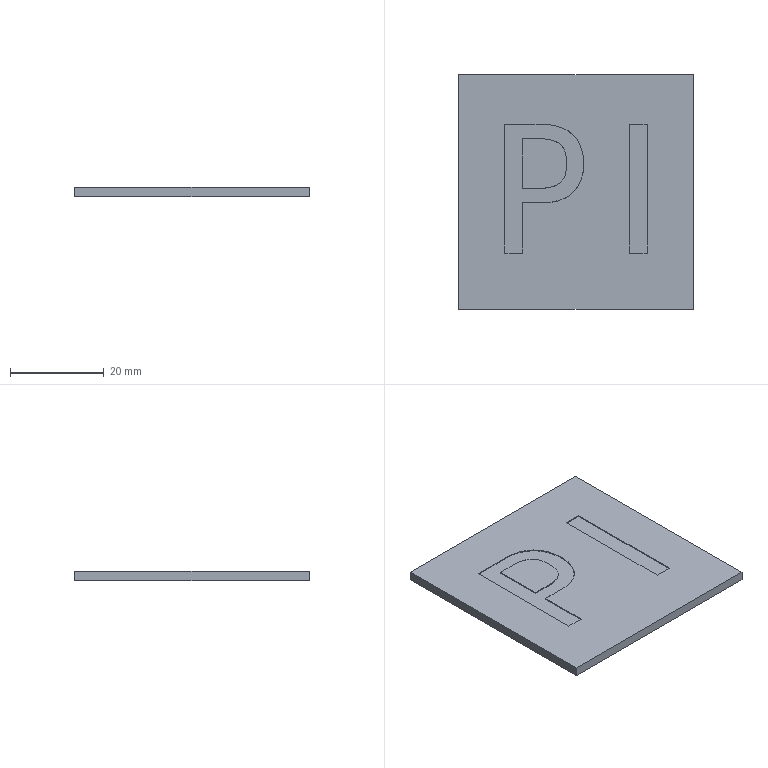Part | STEP file | lll_id1606_x_t | 1 solid | 21 faces | box 50 x 50 x 2 mm | volume 4939 mm3 | plane 17 | other 4
STEP:
#1=CARTESIAN_POINT('',(3595.876,-531.694,3.259));
#2=VERTEX_POINT('',#1);
#3=CARTESIAN_POINT('',(3610.45,-533.931,3.259));
#4=VERTEX_POINT('',#3);
#5=CARTESIAN_POINT('',(3595.876,-531.694,3.259));
#6=CARTESIAN_POINT('',(3598.652,-531.694,3.259));
#7=CARTESIAN_POINT('',(3601.429,-531.694,3.259));
#8=CARTESIAN_POINT('',(3606.87,-531.694,3.259));
#9=CARTESIAN_POINT('',(3608.949,-532.437,3.259));
#10=CARTESIAN_POINT('',(3610.45,-533.931,3.259));
#11=B_SPLINE_CURVE_WITH_KNOTS('',3,(#5,#6,#7,#8,#9,#10),.UNSPECIFIED.,.F.,.F.,(4,2,4),(0.,0.5103,1.),.UNSPECIFIED.);
#12=EDGE_CURVE('',#2,#4,#11,.T.);
#13=ORIENTED_EDGE('',*,*,#12,.T.);
#14=CARTESIAN_POINT('',(3599.561,-548.34,3.259));
#15=VERTEX_POINT('',#14);
#16=CARTESIAN_POINT('',(3610.45,-533.931,3.259));
#17=CARTESIAN_POINT('',(3611.944,-535.424,3.259));
#18=CARTESIAN_POINT('',(3612.687,-537.458,3.259));
#19=CARTESIAN_POINT('',(3612.687,-542.576,3.259));
#20=CARTESIAN_POINT('',(3611.944,-544.603,3.259));
#21=CARTESIAN_POINT('',(3608.957,-547.605,3.259));
#22=CARTESIAN_POINT('',(3606.87,-548.34,3.259));
#23=CARTESIAN_POINT('',(3602.658,-548.34,3.259));
#24=CARTESIAN_POINT('',(3601.109,-548.34,3.259));
#25=CARTESIAN_POINT('',(3599.561,-548.34,3.259));
#26=B_SPLINE_CURVE_WITH_KNOTS('',3,(#16,#17,#18,#19,#20,#21,#22,#23,#24,#25),.UNSPECIFIED.,.F.,.F.,(4,2,2,2,4),(0.,0.2792,0.5585,0.8377,1.),.UNSPECIFIED.);
#27=EDGE_CURVE('',#4,#15,#26,.T.);
#28=ORIENTED_EDGE('',*,*,#27,.T.);
#29=CARTESIAN_POINT('',(3599.561,-559.065,3.259));
#30=VERTEX_POINT('',#29);
#31=CARTESIAN_POINT('',(3599.561,-553.703,3.259));
#32=DIRECTION('',(0.,-1.,0.));
#33=VECTOR('',#32,1.);
#34=LINE('',#31,#33);
#35=EDGE_CURVE('',#15,#30,#34,.T.);
#36=ORIENTED_EDGE('',*,*,#35,.T.);
#37=CARTESIAN_POINT('',(3595.876,-559.065,3.259));
#38=VERTEX_POINT('',#37);
#39=CARTESIAN_POINT('',(3597.718,-559.065,3.259));
#40=DIRECTION('',(-1.,0.,0.));
#41=VECTOR('',#40,1.);
#42=LINE('',#39,#41);
#43=EDGE_CURVE('',#30,#38,#42,.T.);
#44=ORIENTED_EDGE('',*,*,#43,.T.);
#45=CARTESIAN_POINT('',(3595.876,-545.38,3.259));
#46=DIRECTION('',(0.,1.,0.));
#47=VECTOR('',#46,1.);
#48=LINE('',#45,#47);
#49=EDGE_CURVE('',#38,#2,#48,.T.);
#50=ORIENTED_EDGE('',*,*,#49,.T.);
#51=EDGE_LOOP('',(#13,#28,#36,#44,#50));
#52=FACE_BOUND('',#51,.T.);
#53=CARTESIAN_POINT('',(3586.009,-571.065,3.259));
#54=VERTEX_POINT('',#53);
#55=CARTESIAN_POINT('',(3586.009,-521.065,3.259));
#56=VERTEX_POINT('',#55);
#57=CARTESIAN_POINT('',(3586.009,-471.065,3.259));
#58=DIRECTION('',(0.,1.,0.));
#59=VECTOR('',#58,1.);
#60=LINE('',#57,#59);
#61=EDGE_CURVE('',#54,#56,#60,.T.);
#62=ORIENTED_EDGE('',*,*,#61,.F.);
#63=CARTESIAN_POINT('',(3636.009,-571.065,3.259));
#64=VERTEX_POINT('',#63);
#65=CARTESIAN_POINT('',(3636.009,-571.065,3.259));
#66=DIRECTION('',(-1.,0.,0.));
#67=VECTOR('',#66,1.);
#68=LINE('',#65,#67);
#69=EDGE_CURVE('',#64,#54,#68,.T.);
#70=ORIENTED_EDGE('',*,*,#69,.F.);
#71=CARTESIAN_POINT('',(3636.009,-521.065,3.259));
#72=VERTEX_POINT('',#71);
#73=CARTESIAN_POINT('',(3636.009,-471.065,3.259));
#74=DIRECTION('',(0.,-1.,0.));
#75=VECTOR('',#74,1.);
#76=LINE('',#73,#75);
#77=EDGE_CURVE('',#72,#64,#76,.T.);
#78=ORIENTED_EDGE('',*,*,#77,.F.);
#79=CARTESIAN_POINT('',(3636.009,-521.065,3.259));
#80=DIRECTION('',(-1.,0.,0.));
#81=VECTOR('',#80,1.);
#82=LINE('',#79,#81);
#83=EDGE_CURVE('',#72,#56,#82,.T.);
#84=ORIENTED_EDGE('',*,*,#83,.T.);
#85=EDGE_LOOP('',(#62,#70,#78,#84));
#86=FACE_BOUND('',#85,.T.);
#87=CARTESIAN_POINT('',(3622.458,-531.694,3.259));
#88=VERTEX_POINT('',#87);
#89=CARTESIAN_POINT('',(3626.143,-531.694,3.259));
#90=VERTEX_POINT('',#89);
#91=CARTESIAN_POINT('',(3624.301,-531.694,3.259));
#92=DIRECTION('',(1.,0.,0.));
#93=VECTOR('',#92,1.);
#94=LINE('',#91,#93);
#95=EDGE_CURVE('',#88,#90,#94,.T.);
#96=ORIENTED_EDGE('',*,*,#95,.T.);
#97=CARTESIAN_POINT('',(3626.143,-559.065,3.259));
#98=VERTEX_POINT('',#97);
#99=CARTESIAN_POINT('',(3626.143,-545.38,3.259));
#100=DIRECTION('',(0.,-1.,0.));
#101=VECTOR('',#100,1.);
#102=LINE('',#99,#101);
#103=EDGE_CURVE('',#90,#98,#102,.T.);
#104=ORIENTED_EDGE('',*,*,#103,.T.);
#105=CARTESIAN_POINT('',(3622.458,-559.065,3.259));
#106=VERTEX_POINT('',#105);
#107=CARTESIAN_POINT('',(3624.301,-559.065,3.259));
#108=DIRECTION('',(-1.,0.,0.));
#109=VECTOR('',#108,1.);
#110=LINE('',#107,#109);
#111=EDGE_CURVE('',#98,#106,#110,.T.);
#112=ORIENTED_EDGE('',*,*,#111,.T.);
#113=CARTESIAN_POINT('',(3622.458,-545.38,3.259));
#114=DIRECTION('',(0.,1.,0.));
#115=VECTOR('',#114,1.);
#116=LINE('',#113,#115);
#117=EDGE_CURVE('',#106,#88,#116,.T.);
#118=ORIENTED_EDGE('',*,*,#117,.T.);
#119=EDGE_LOOP('',(#96,#104,#112,#118));
#120=FACE_BOUND('',#119,.T.);
#121=CARTESIAN_POINT('',(3636.009,-471.065,3.259));
#122=DIRECTION('',(0.,0.,1.));
#123=DIRECTION('',(1.,0.,0.));
#124=AXIS2_PLACEMENT_3D('',#121,#122,#123);
#125=PLANE('',#124);
#126=ADVANCED_FACE('',(#52,#86,#120),#125,.T.);
#127=CARTESIAN_POINT('',(3586.009,-571.065,1.259));
#128=VERTEX_POINT('',#127);
#129=CARTESIAN_POINT('',(3586.009,-521.065,1.259));
#130=VERTEX_POINT('',#129);
#131=CARTESIAN_POINT('',(3586.009,-471.065,1.259));
#132=DIRECTION('',(0.,1.,0.));
#133=VECTOR('',#132,1.);
#134=LINE('',#131,#133);
#135=EDGE_CURVE('',#128,#130,#134,.T.);
#136=ORIENTED_EDGE('',*,*,#135,.T.);
#137=CARTESIAN_POINT('',(3636.009,-521.065,1.259));
#138=VERTEX_POINT('',#137);
#139=CARTESIAN_POINT('',(2076.009,-521.065,1.259));
#140=DIRECTION('',(1.,0.,0.));
#141=VECTOR('',#140,1.);
#142=LINE('',#139,#141);
#143=EDGE_CURVE('',#130,#138,#142,.T.);
#144=ORIENTED_EDGE('',*,*,#143,.T.);
#145=CARTESIAN_POINT('',(3636.009,-571.065,1.259));
#146=VERTEX_POINT('',#145);
#147=CARTESIAN_POINT('',(3636.009,-471.065,1.259));
#148=DIRECTION('',(0.,-1.,0.));
#149=VECTOR('',#148,1.);
#150=LINE('',#147,#149);
#151=EDGE_CURVE('',#138,#146,#150,.T.);
#152=ORIENTED_EDGE('',*,*,#151,.T.);
#153=CARTESIAN_POINT('',(-3680.12,-571.065,1.259));
#154=DIRECTION('',(1.,0.,0.));
#155=VECTOR('',#154,1.);
#156=LINE('',#153,#155);
#157=EDGE_CURVE('',#128,#146,#156,.T.);
#158=ORIENTED_EDGE('',*,*,#157,.F.);
#159=EDGE_LOOP('',(#136,#144,#152,#158));
#160=FACE_OUTER_BOUND('',#159,.T.);
#161=CARTESIAN_POINT('',(2076.009,-471.065,1.259));
#162=DIRECTION('',(0.,0.,-1.));
#163=DIRECTION('',(-1.,0.,0.));
#164=AXIS2_PLACEMENT_3D('',#161,#162,#163);
#165=PLANE('',#164);
#166=ADVANCED_FACE('',(#160),#165,.T.);
#167=ORIENTED_EDGE('',*,*,#151,.F.);
#168=CARTESIAN_POINT('',(3636.009,-521.065,0.9594));
#169=DIRECTION('',(0.,0.,-1.));
#170=VECTOR('',#169,1.);
#171=LINE('',#168,#170);
#172=EDGE_CURVE('',#72,#138,#171,.T.);
#173=ORIENTED_EDGE('',*,*,#172,.F.);
#174=ORIENTED_EDGE('',*,*,#77,.T.);
#175=CARTESIAN_POINT('',(3636.009,-571.065,0.9594));
#176=DIRECTION('',(0.,0.,1.));
#177=VECTOR('',#176,1.);
#178=LINE('',#175,#177);
#179=EDGE_CURVE('',#146,#64,#178,.T.);
#180=ORIENTED_EDGE('',*,*,#179,.F.);
#181=EDGE_LOOP('',(#167,#173,#174,#180));
#182=FACE_OUTER_BOUND('',#181,.T.);
#183=CARTESIAN_POINT('',(3636.009,-471.065,0.9594));
#184=DIRECTION('',(1.,0.,0.));
#185=DIRECTION('',(0.,0.,-1.));
#186=AXIS2_PLACEMENT_3D('',#183,#184,#185);
#187=PLANE('',#186);
#188=ADVANCED_FACE('',(#182),#187,.T.);
#189=CARTESIAN_POINT('',(3586.009,-571.065,179.534));
#190=DIRECTION('',(0.,0.,-1.));
#191=VECTOR('',#190,1.);
#192=LINE('',#189,#191);
#193=EDGE_CURVE('',#54,#128,#192,.T.);
#194=ORIENTED_EDGE('',*,*,#193,.T.);
#195=ORIENTED_EDGE('',*,*,#157,.T.);
#196=ORIENTED_EDGE('',*,*,#179,.T.);
#197=ORIENTED_EDGE('',*,*,#69,.T.);
#198=EDGE_LOOP('',(#194,#195,#196,#197));
#199=FACE_OUTER_BOUND('',#198,.T.);
#200=CARTESIAN_POINT('',(-3680.12,-571.065,179.534));
#201=DIRECTION('',(0.,-1.,0.));
#202=DIRECTION('',(0.,0.,-1.));
#203=AXIS2_PLACEMENT_3D('',#200,#201,#202);
#204=PLANE('',#203);
#205=ADVANCED_FACE('',(#199),#204,.T.);
#206=CARTESIAN_POINT('',(3586.009,-521.065,2.109));
#207=DIRECTION('',(0.,0.,1.));
#208=VECTOR('',#207,1.);
#209=LINE('',#206,#208);
#210=EDGE_CURVE('',#130,#56,#209,.T.);
#211=ORIENTED_EDGE('',*,*,#210,.T.);
#212=ORIENTED_EDGE('',*,*,#83,.F.);
#213=ORIENTED_EDGE('',*,*,#172,.T.);
#214=ORIENTED_EDGE('',*,*,#143,.F.);
#215=EDGE_LOOP('',(#211,#212,#213,#214));
#216=FACE_OUTER_BOUND('',#215,.T.);
#217=CARTESIAN_POINT('',(3586.009,-521.065,2.109));
#218=DIRECTION('',(0.,1.,0.));
#219=DIRECTION('',(0.,0.,1.));
#220=AXIS2_PLACEMENT_3D('',#217,#218,#219);
#221=PLANE('',#220);
#222=ADVANCED_FACE('',(#216),#221,.T.);
#223=ORIENTED_EDGE('',*,*,#193,.F.);
#224=ORIENTED_EDGE('',*,*,#61,.T.);
#225=ORIENTED_EDGE('',*,*,#210,.F.);
#226=ORIENTED_EDGE('',*,*,#135,.F.);
#227=EDGE_LOOP('',(#223,#224,#225,#226));
#228=FACE_OUTER_BOUND('',#227,.T.);
#229=CARTESIAN_POINT('',(3586.009,-546.065,2.259));
#230=DIRECTION('',(1.,0.,0.));
#231=DIRECTION('',(0.,0.,-1.));
#232=AXIS2_PLACEMENT_3D('',#229,#230,#231);
#233=PLANE('',#232);
#234=ADVANCED_FACE('',(#228),#233,.F.);
#235=CARTESIAN_POINT('',(3607.568,-544.182,3.259));
#236=VERTEX_POINT('',#235);
#237=CARTESIAN_POINT('',(3599.561,-534.734,3.259));
#238=VERTEX_POINT('',#237);
#239=CARTESIAN_POINT('',(3607.568,-544.182,3.259));
#240=CARTESIAN_POINT('',(3608.529,-543.432,3.259));
#241=CARTESIAN_POINT('',(3609.009,-542.044,3.259));
#242=CARTESIAN_POINT('',(3609.009,-537.991,3.259));
#243=CARTESIAN_POINT('',(3608.529,-536.602,3.259));
#244=CARTESIAN_POINT('',(3606.611,-535.104,3.259));
#245=CARTESIAN_POINT('',(3605.167,-534.734,3.259));
#246=CARTESIAN_POINT('',(3602.017,-534.734,3.259));
#247=CARTESIAN_POINT('',(3600.789,-534.734,3.259));
#248=CARTESIAN_POINT('',(3599.561,-534.734,3.259));
#249=B_SPLINE_CURVE_WITH_KNOTS('',3,(#239,#240,#241,#242,#243,#244,#245,#246,#247,#248),.UNSPECIFIED.,.F.,.F.,(4,2,2,2,4),(0.,0.2752,0.5505,0.8247,1.),.UNSPECIFIED.);
#250=EDGE_CURVE('',#236,#238,#249,.T.);
#251=ORIENTED_EDGE('',*,*,#250,.F.);
#252=CARTESIAN_POINT('',(3607.568,-544.182,3.059));
#253=VERTEX_POINT('',#252);
#254=CARTESIAN_POINT('',(3607.568,-544.182,3.059));
#255=DIRECTION('',(0.,0.,-1.));
#256=VECTOR('',#255,1.);
#257=LINE('',#254,#256);
#258=EDGE_CURVE('',#236,#253,#257,.T.);
#259=ORIENTED_EDGE('',*,*,#258,.T.);
#260=CARTESIAN_POINT('',(3599.561,-534.734,3.059));
#261=VERTEX_POINT('',#260);
#262=CARTESIAN_POINT('',(3599.561,-534.734,3.059));
#263=CARTESIAN_POINT('',(3600.789,-534.734,3.059));
#264=CARTESIAN_POINT('',(3602.017,-534.734,3.059));
#265=CARTESIAN_POINT('',(3605.167,-534.734,3.059));
#266=CARTESIAN_POINT('',(3606.611,-535.104,3.059));
#267=CARTESIAN_POINT('',(3608.529,-536.602,3.059));
#268=CARTESIAN_POINT('',(3609.009,-537.991,3.059));
#269=CARTESIAN_POINT('',(3609.009,-542.044,3.059));
#270=CARTESIAN_POINT('',(3608.529,-543.432,3.059));
#271=CARTESIAN_POINT('',(3607.568,-544.182,3.059));
#272=B_SPLINE_CURVE_WITH_KNOTS('',3,(#262,#263,#264,#265,#266,#267,#268,#269,#270,#271),.UNSPECIFIED.,.F.,.F.,(4,2,2,2,4),(0.,0.1753,0.4495,0.7248,1.),.UNSPECIFIED.);
#273=EDGE_CURVE('',#261,#253,#272,.T.);
#274=ORIENTED_EDGE('',*,*,#273,.F.);
#275=CARTESIAN_POINT('',(3599.561,-534.734,3.059));
#276=DIRECTION('',(0.,0.,-1.));
#277=VECTOR('',#276,1.);
#278=LINE('',#275,#277);
#279=EDGE_CURVE('',#238,#261,#278,.T.);
#280=ORIENTED_EDGE('',*,*,#279,.F.);
#281=EDGE_LOOP('',(#251,#259,#274,#280));
#282=FACE_OUTER_BOUND('',#281,.T.);
#283=CARTESIAN_POINT('',(3607.568,-544.182,3.059));
#284=CARTESIAN_POINT('',(3608.529,-543.432,3.059));
#285=CARTESIAN_POINT('',(3609.009,-542.044,3.059));
#286=CARTESIAN_POINT('',(3609.009,-537.991,3.059));
#287=CARTESIAN_POINT('',(3608.529,-536.602,3.059));
#288=CARTESIAN_POINT('',(3606.611,-535.104,3.059));
#289=CARTESIAN_POINT('',(3605.167,-534.734,3.059));
#290=CARTESIAN_POINT('',(3602.017,-534.734,3.059));
#291=CARTESIAN_POINT('',(3600.789,-534.734,3.059));
#292=CARTESIAN_POINT('',(3599.561,-534.734,3.059));
#293=B_SPLINE_CURVE_WITH_KNOTS('',3,(#283,#284,#285,#286,#287,#288,#289,#290,#291,#292),.UNSPECIFIED.,.F.,.F.,(4,2,2,2,4),(0.,0.2752,0.5505,0.8247,1.),.UNSPECIFIED.);
#294=DIRECTION('',(0.,0.,1.));
#295=VECTOR('',#294,1.);
#296=SURFACE_OF_LINEAR_EXTRUSION('',#293,#295);
#297=ADVANCED_FACE('',(#282),#296,.T.);
#298=CARTESIAN_POINT('',(3599.561,-545.301,3.259));
#299=VERTEX_POINT('',#298);
#300=CARTESIAN_POINT('',(3599.561,-540.017,3.259));
#301=DIRECTION('',(0.,-1.,0.));
#302=VECTOR('',#301,1.);
#303=LINE('',#300,#302);
#304=EDGE_CURVE('',#238,#299,#303,.T.);
#305=ORIENTED_EDGE('',*,*,#304,.F.);
#306=ORIENTED_EDGE('',*,*,#279,.T.);
#307=CARTESIAN_POINT('',(3599.561,-545.301,3.059));
#308=VERTEX_POINT('',#307);
#309=CARTESIAN_POINT('',(3599.561,-540.017,3.059));
#310=DIRECTION('',(0.,1.,0.));
#311=VECTOR('',#310,1.);
#312=LINE('',#309,#311);
#313=EDGE_CURVE('',#308,#261,#312,.T.);
#314=ORIENTED_EDGE('',*,*,#313,.F.);
#315=CARTESIAN_POINT('',(3599.561,-545.301,3.059));
#316=DIRECTION('',(0.,0.,-1.));
#317=VECTOR('',#316,1.);
#318=LINE('',#315,#317);
#319=EDGE_CURVE('',#299,#308,#318,.T.);
#320=ORIENTED_EDGE('',*,*,#319,.F.);
#321=EDGE_LOOP('',(#305,#306,#314,#320));
#322=FACE_OUTER_BOUND('',#321,.T.);
#323=CARTESIAN_POINT('',(3599.561,-534.734,3.059));
#324=DIRECTION('',(-1.,0.,0.));
#325=DIRECTION('',(0.,0.,1.));
#326=AXIS2_PLACEMENT_3D('',#323,#324,#325);
#327=PLANE('',#326);
#328=ADVANCED_FACE('',(#322),#327,.T.);
#329=ORIENTED_EDGE('',*,*,#27,.F.);
#330=CARTESIAN_POINT('',(3610.45,-533.931,3.059));
#331=VERTEX_POINT('',#330);
#332=CARTESIAN_POINT('',(3610.45,-533.931,3.059));
#333=DIRECTION('',(0.,0.,-1.));
#334=VECTOR('',#333,1.);
#335=LINE('',#332,#334);
#336=EDGE_CURVE('',#4,#331,#335,.T.);
#337=ORIENTED_EDGE('',*,*,#336,.T.);
#338=CARTESIAN_POINT('',(3599.561,-548.34,3.059));
#339=VERTEX_POINT('',#338);
#340=CARTESIAN_POINT('',(3599.561,-548.34,3.059));
#341=CARTESIAN_POINT('',(3601.109,-548.34,3.059));
#342=CARTESIAN_POINT('',(3602.658,-548.34,3.059));
#343=CARTESIAN_POINT('',(3606.87,-548.34,3.059));
#344=CARTESIAN_POINT('',(3608.957,-547.605,3.059));
#345=CARTESIAN_POINT('',(3611.944,-544.603,3.059));
#346=CARTESIAN_POINT('',(3612.687,-542.576,3.059));
#347=CARTESIAN_POINT('',(3612.687,-537.458,3.059));
#348=CARTESIAN_POINT('',(3611.944,-535.424,3.059));
#349=CARTESIAN_POINT('',(3610.45,-533.931,3.059));
#350=B_SPLINE_CURVE_WITH_KNOTS('',3,(#340,#341,#342,#343,#344,#345,#346,#347,#348,#349),.UNSPECIFIED.,.F.,.F.,(4,2,2,2,4),(0.,0.1623,0.4415,0.7208,1.),.UNSPECIFIED.);
#351=EDGE_CURVE('',#339,#331,#350,.T.);
#352=ORIENTED_EDGE('',*,*,#351,.F.);
#353=CARTESIAN_POINT('',(3599.561,-548.34,3.059));
#354=DIRECTION('',(0.,0.,-1.));
#355=VECTOR('',#354,1.);
#356=LINE('',#353,#355);
#357=EDGE_CURVE('',#15,#339,#356,.T.);
#358=ORIENTED_EDGE('',*,*,#357,.F.);
#359=EDGE_LOOP('',(#329,#337,#352,#358));
#360=FACE_OUTER_BOUND('',#359,.T.);
#361=CARTESIAN_POINT('',(3610.45,-533.931,3.059));
#362=CARTESIAN_POINT('',(3611.944,-535.424,3.059));
#363=CARTESIAN_POINT('',(3612.687,-537.458,3.059));
#364=CARTESIAN_POINT('',(3612.687,-542.576,3.059));
#365=CARTESIAN_POINT('',(3611.944,-544.603,3.059));
#366=CARTESIAN_POINT('',(3608.957,-547.605,3.059));
#367=CARTESIAN_POINT('',(3606.87,-548.34,3.059));
#368=CARTESIAN_POINT('',(3602.658,-548.34,3.059));
#369=CARTESIAN_POINT('',(3601.109,-548.34,3.059));
#370=CARTESIAN_POINT('',(3599.561,-548.34,3.059));
#371=B_SPLINE_CURVE_WITH_KNOTS('',3,(#361,#362,#363,#364,#365,#366,#367,#368,#369,#370),.UNSPECIFIED.,.F.,.F.,(4,2,2,2,4),(0.,0.2792,0.5585,0.8377,1.),.UNSPECIFIED.);
#372=DIRECTION('',(0.,0.,1.));
#373=VECTOR('',#372,1.);
#374=SURFACE_OF_LINEAR_EXTRUSION('',#371,#373);
#375=ADVANCED_FACE('',(#360),#374,.T.);
#376=ORIENTED_EDGE('',*,*,#35,.F.);
#377=ORIENTED_EDGE('',*,*,#357,.T.);
#378=CARTESIAN_POINT('',(3599.561,-559.065,3.059));
#379=VERTEX_POINT('',#378);
#380=CARTESIAN_POINT('',(3599.561,-553.703,3.059));
#381=DIRECTION('',(0.,1.,0.));
#382=VECTOR('',#381,1.);
#383=LINE('',#380,#382);
#384=EDGE_CURVE('',#379,#339,#383,.T.);
#385=ORIENTED_EDGE('',*,*,#384,.F.);
#386=CARTESIAN_POINT('',(3599.561,-559.065,3.059));
#387=DIRECTION('',(0.,0.,-1.));
#388=VECTOR('',#387,1.);
#389=LINE('',#386,#388);
#390=EDGE_CURVE('',#30,#379,#389,.T.);
#391=ORIENTED_EDGE('',*,*,#390,.F.);
#392=EDGE_LOOP('',(#376,#377,#385,#391));
#393=FACE_OUTER_BOUND('',#392,.T.);
#394=CARTESIAN_POINT('',(3599.561,-548.34,3.059));
#395=DIRECTION('',(-1.,0.,0.));
#396=DIRECTION('',(0.,0.,1.));
#397=AXIS2_PLACEMENT_3D('',#394,#395,#396);
#398=PLANE('',#397);
#399=ADVANCED_FACE('',(#393),#398,.T.);
#400=ORIENTED_EDGE('',*,*,#43,.F.);
#401=ORIENTED_EDGE('',*,*,#390,.T.);
#402=CARTESIAN_POINT('',(3595.876,-559.065,3.059));
#403=VERTEX_POINT('',#402);
#404=CARTESIAN_POINT('',(3597.718,-559.065,3.059));
#405=DIRECTION('',(1.,0.,0.));
#406=VECTOR('',#405,1.);
#407=LINE('',#404,#406);
#408=EDGE_CURVE('',#403,#379,#407,.T.);
#409=ORIENTED_EDGE('',*,*,#408,.F.);
#410=CARTESIAN_POINT('',(3595.876,-559.065,3.059));
#411=DIRECTION('',(0.,0.,-1.));
#412=VECTOR('',#411,1.);
#413=LINE('',#410,#412);
#414=EDGE_CURVE('',#38,#403,#413,.T.);
#415=ORIENTED_EDGE('',*,*,#414,.F.);
#416=EDGE_LOOP('',(#400,#401,#409,#415));
#417=FACE_OUTER_BOUND('',#416,.T.);
#418=CARTESIAN_POINT('',(3599.561,-559.065,3.059));
#419=DIRECTION('',(0.,1.,0.));
#420=DIRECTION('',(0.,0.,1.));
#421=AXIS2_PLACEMENT_3D('',#418,#419,#420);
#422=PLANE('',#421);
#423=ADVANCED_FACE('',(#417),#422,.T.);
#424=ORIENTED_EDGE('',*,*,#49,.F.);
#425=ORIENTED_EDGE('',*,*,#414,.T.);
#426=CARTESIAN_POINT('',(3595.876,-531.694,3.059));
#427=VERTEX_POINT('',#426);
#428=CARTESIAN_POINT('',(3595.876,-545.38,3.059));
#429=DIRECTION('',(0.,-1.,0.));
#430=VECTOR('',#429,1.);
#431=LINE('',#428,#430);
#432=EDGE_CURVE('',#427,#403,#431,.T.);
#433=ORIENTED_EDGE('',*,*,#432,.F.);
#434=CARTESIAN_POINT('',(3595.876,-531.694,3.059));
#435=DIRECTION('',(0.,0.,-1.));
#436=VECTOR('',#435,1.);
#437=LINE('',#434,#436);
#438=EDGE_CURVE('',#2,#427,#437,.T.);
#439=ORIENTED_EDGE('',*,*,#438,.F.);
#440=EDGE_LOOP('',(#424,#425,#433,#439));
#441=FACE_OUTER_BOUND('',#440,.T.);
#442=CARTESIAN_POINT('',(3595.876,-559.065,3.059));
#443=DIRECTION('',(1.,0.,0.));
#444=DIRECTION('',(0.,0.,-1.));
#445=AXIS2_PLACEMENT_3D('',#442,#443,#444);
#446=PLANE('',#445);
#447=ADVANCED_FACE('',(#441),#446,.T.);
#448=ORIENTED_EDGE('',*,*,#12,.F.);
#449=ORIENTED_EDGE('',*,*,#438,.T.);
#450=CARTESIAN_POINT('',(3610.45,-533.931,3.059));
#451=CARTESIAN_POINT('',(3608.949,-532.437,3.059));
#452=CARTESIAN_POINT('',(3606.87,-531.694,3.059));
#453=CARTESIAN_POINT('',(3601.429,-531.694,3.059));
#454=CARTESIAN_POINT('',(3598.652,-531.694,3.059));
#455=CARTESIAN_POINT('',(3595.876,-531.694,3.059));
#456=B_SPLINE_CURVE_WITH_KNOTS('',3,(#450,#451,#452,#453,#454,#455),.UNSPECIFIED.,.F.,.F.,(4,2,4),(0.,0.4897,1.),.UNSPECIFIED.);
#457=EDGE_CURVE('',#331,#427,#456,.T.);
#458=ORIENTED_EDGE('',*,*,#457,.F.);
#459=ORIENTED_EDGE('',*,*,#336,.F.);
#460=EDGE_LOOP('',(#448,#449,#458,#459));
#461=FACE_OUTER_BOUND('',#460,.T.);
#462=CARTESIAN_POINT('',(3595.876,-531.694,3.059));
#463=CARTESIAN_POINT('',(3598.652,-531.694,3.059));
#464=CARTESIAN_POINT('',(3601.429,-531.694,3.059));
#465=CARTESIAN_POINT('',(3606.87,-531.694,3.059));
#466=CARTESIAN_POINT('',(3608.949,-532.437,3.059));
#467=CARTESIAN_POINT('',(3610.45,-533.931,3.059));
#468=B_SPLINE_CURVE_WITH_KNOTS('',3,(#462,#463,#464,#465,#466,#467),.UNSPECIFIED.,.F.,.F.,(4,2,4),(0.,0.5103,1.),.UNSPECIFIED.);
#469=DIRECTION('',(0.,0.,1.));
#470=VECTOR('',#469,1.);
#471=SURFACE_OF_LINEAR_EXTRUSION('',#468,#470);
#472=ADVANCED_FACE('',(#461),#471,.T.);
#473=CARTESIAN_POINT('',(3599.561,-545.301,3.259));
#474=CARTESIAN_POINT('',(3600.789,-545.301,3.259));
#475=CARTESIAN_POINT('',(3602.017,-545.301,3.259));
#476=CARTESIAN_POINT('',(3605.167,-545.301,3.259));
#477=CARTESIAN_POINT('',(3606.608,-544.925,3.259));
#478=CARTESIAN_POINT('',(3607.568,-544.182,3.259));
#479=B_SPLINE_CURVE_WITH_KNOTS('',3,(#473,#474,#475,#476,#477,#478),.UNSPECIFIED.,.F.,.F.,(4,2,4),(0.,0.39,1.),.UNSPECIFIED.);
#480=EDGE_CURVE('',#299,#236,#479,.T.);
#481=ORIENTED_EDGE('',*,*,#480,.F.);
#482=ORIENTED_EDGE('',*,*,#319,.T.);
#483=CARTESIAN_POINT('',(3607.568,-544.182,3.059));
#484=CARTESIAN_POINT('',(3606.608,-544.925,3.059));
#485=CARTESIAN_POINT('',(3605.167,-545.301,3.059));
#486=CARTESIAN_POINT('',(3602.017,-545.301,3.059));
#487=CARTESIAN_POINT('',(3600.789,-545.301,3.059));
#488=CARTESIAN_POINT('',(3599.561,-545.301,3.059));
#489=B_SPLINE_CURVE_WITH_KNOTS('',3,(#483,#484,#485,#486,#487,#488),.UNSPECIFIED.,.F.,.F.,(4,2,4),(0.,0.61,1.),.UNSPECIFIED.);
#490=EDGE_CURVE('',#253,#308,#489,.T.);
#491=ORIENTED_EDGE('',*,*,#490,.F.);
#492=ORIENTED_EDGE('',*,*,#258,.F.);
#493=EDGE_LOOP('',(#481,#482,#491,#492));
#494=FACE_OUTER_BOUND('',#493,.T.);
#495=CARTESIAN_POINT('',(3599.561,-545.301,3.059));
#496=CARTESIAN_POINT('',(3600.789,-545.301,3.059));
#497=CARTESIAN_POINT('',(3602.017,-545.301,3.059));
#498=CARTESIAN_POINT('',(3605.167,-545.301,3.059));
#499=CARTESIAN_POINT('',(3606.608,-544.925,3.059));
#500=CARTESIAN_POINT('',(3607.568,-544.182,3.059));
#501=B_SPLINE_CURVE_WITH_KNOTS('',3,(#495,#496,#497,#498,#499,#500),.UNSPECIFIED.,.F.,.F.,(4,2,4),(0.,0.39,1.),.UNSPECIFIED.);
#502=DIRECTION('',(0.,0.,1.));
#503=VECTOR('',#502,1.);
#504=SURFACE_OF_LINEAR_EXTRUSION('',#501,#503);
#505=ADVANCED_FACE('',(#494),#504,.T.);
#506=ORIENTED_EDGE('',*,*,#351,.T.);
#507=ORIENTED_EDGE('',*,*,#457,.T.);
#508=ORIENTED_EDGE('',*,*,#432,.T.);
#509=ORIENTED_EDGE('',*,*,#408,.T.);
#510=ORIENTED_EDGE('',*,*,#384,.T.);
#511=EDGE_LOOP('',(#506,#507,#508,#509,#510));
#512=FACE_BOUND('',#511,.T.);
#513=ORIENTED_EDGE('',*,*,#273,.T.);
#514=ORIENTED_EDGE('',*,*,#490,.T.);
#515=ORIENTED_EDGE('',*,*,#313,.T.);
#516=EDGE_LOOP('',(#513,#514,#515));
#517=FACE_BOUND('',#516,.T.);
#518=CARTESIAN_POINT('',(3611.29,-545.092,3.059));
#519=DIRECTION('',(0.,0.,1.));
#520=DIRECTION('',(1.,0.,0.));
#521=AXIS2_PLACEMENT_3D('',#518,#519,#520);
#522=PLANE('',#521);
#523=ADVANCED_FACE('',(#512,#517),#522,.T.);
#524=ORIENTED_EDGE('',*,*,#480,.T.);
#525=ORIENTED_EDGE('',*,*,#250,.T.);
#526=ORIENTED_EDGE('',*,*,#304,.T.);
#527=EDGE_LOOP('',(#524,#525,#526));
#528=FACE_OUTER_BOUND('',#527,.T.);
#529=CARTESIAN_POINT('',(3636.009,-471.065,3.259));
#530=DIRECTION('',(0.,0.,1.));
#531=DIRECTION('',(1.,0.,0.));
#532=AXIS2_PLACEMENT_3D('',#529,#530,#531);
#533=PLANE('',#532);
#534=ADVANCED_FACE('',(#528),#533,.T.);
#535=ORIENTED_EDGE('',*,*,#103,.F.);
#536=CARTESIAN_POINT('',(3626.143,-531.694,3.059));
#537=VERTEX_POINT('',#536);
#538=CARTESIAN_POINT('',(3626.143,-531.694,3.059));
#539=DIRECTION('',(0.,0.,-1.));
#540=VECTOR('',#539,1.);
#541=LINE('',#538,#540);
#542=EDGE_CURVE('',#90,#537,#541,.T.);
#543=ORIENTED_EDGE('',*,*,#542,.T.);
#544=CARTESIAN_POINT('',(3626.143,-559.065,3.059));
#545=VERTEX_POINT('',#544);
#546=CARTESIAN_POINT('',(3626.143,-545.38,3.059));
#547=DIRECTION('',(0.,1.,0.));
#548=VECTOR('',#547,1.);
#549=LINE('',#546,#548);
#550=EDGE_CURVE('',#545,#537,#549,.T.);
#551=ORIENTED_EDGE('',*,*,#550,.F.);
#552=CARTESIAN_POINT('',(3626.143,-559.065,3.059));
#553=DIRECTION('',(0.,0.,-1.));
#554=VECTOR('',#553,1.);
#555=LINE('',#552,#554);
#556=EDGE_CURVE('',#98,#545,#555,.T.);
#557=ORIENTED_EDGE('',*,*,#556,.F.);
#558=EDGE_LOOP('',(#535,#543,#551,#557));
#559=FACE_OUTER_BOUND('',#558,.T.);
#560=CARTESIAN_POINT('',(3626.143,-531.694,3.059));
#561=DIRECTION('',(-1.,0.,0.));
#562=DIRECTION('',(0.,0.,1.));
#563=AXIS2_PLACEMENT_3D('',#560,#561,#562);
#564=PLANE('',#563);
#565=ADVANCED_FACE('',(#559),#564,.T.);
#566=ORIENTED_EDGE('',*,*,#111,.F.);
#567=ORIENTED_EDGE('',*,*,#556,.T.);
#568=CARTESIAN_POINT('',(3622.458,-559.065,3.059));
#569=VERTEX_POINT('',#568);
#570=CARTESIAN_POINT('',(3624.301,-559.065,3.059));
#571=DIRECTION('',(1.,0.,0.));
#572=VECTOR('',#571,1.);
#573=LINE('',#570,#572);
#574=EDGE_CURVE('',#569,#545,#573,.T.);
#575=ORIENTED_EDGE('',*,*,#574,.F.);
#576=CARTESIAN_POINT('',(3622.458,-559.065,3.059));
#577=DIRECTION('',(0.,0.,-1.));
#578=VECTOR('',#577,1.);
#579=LINE('',#576,#578);
#580=EDGE_CURVE('',#106,#569,#579,.T.);
#581=ORIENTED_EDGE('',*,*,#580,.F.);
#582=EDGE_LOOP('',(#566,#567,#575,#581));
#583=FACE_OUTER_BOUND('',#582,.T.);
#584=CARTESIAN_POINT('',(3626.143,-559.065,3.059));
#585=DIRECTION('',(0.,1.,0.));
#586=DIRECTION('',(0.,0.,1.));
#587=AXIS2_PLACEMENT_3D('',#584,#585,#586);
#588=PLANE('',#587);
#589=ADVANCED_FACE('',(#583),#588,.T.);
#590=ORIENTED_EDGE('',*,*,#117,.F.);
#591=ORIENTED_EDGE('',*,*,#580,.T.);
#592=CARTESIAN_POINT('',(3622.458,-531.694,3.059));
#593=VERTEX_POINT('',#592);
#594=CARTESIAN_POINT('',(3622.458,-545.38,3.059));
#595=DIRECTION('',(0.,-1.,0.));
#596=VECTOR('',#595,1.);
#597=LINE('',#594,#596);
#598=EDGE_CURVE('',#593,#569,#597,.T.);
#599=ORIENTED_EDGE('',*,*,#598,.F.);
#600=CARTESIAN_POINT('',(3622.458,-531.694,3.059));
#601=DIRECTION('',(0.,0.,-1.));
#602=VECTOR('',#601,1.);
#603=LINE('',#600,#602);
#604=EDGE_CURVE('',#88,#593,#603,.T.);
#605=ORIENTED_EDGE('',*,*,#604,.F.);
#606=EDGE_LOOP('',(#590,#591,#599,#605));
#607=FACE_OUTER_BOUND('',#606,.T.);
#608=CARTESIAN_POINT('',(3622.458,-559.065,3.059));
#609=DIRECTION('',(1.,0.,0.));
#610=DIRECTION('',(0.,0.,-1.));
#611=AXIS2_PLACEMENT_3D('',#608,#609,#610);
#612=PLANE('',#611);
#613=ADVANCED_FACE('',(#607),#612,.T.);
#614=ORIENTED_EDGE('',*,*,#95,.F.);
#615=ORIENTED_EDGE('',*,*,#604,.T.);
#616=CARTESIAN_POINT('',(3624.301,-531.694,3.059));
#617=DIRECTION('',(-1.,0.,0.));
#618=VECTOR('',#617,1.);
#619=LINE('',#616,#618);
#620=EDGE_CURVE('',#537,#593,#619,.T.);
#621=ORIENTED_EDGE('',*,*,#620,.F.);
#622=ORIENTED_EDGE('',*,*,#542,.F.);
#623=EDGE_LOOP('',(#614,#615,#621,#622));
#624=FACE_OUTER_BOUND('',#623,.T.);
#625=CARTESIAN_POINT('',(3622.458,-531.694,3.059));
#626=DIRECTION('',(0.,-1.,0.));
#627=DIRECTION('',(0.,0.,-1.));
#628=AXIS2_PLACEMENT_3D('',#625,#626,#627);
#629=PLANE('',#628);
#630=ADVANCED_FACE('',(#624),#629,.T.);
#631=ORIENTED_EDGE('',*,*,#550,.T.);
#632=ORIENTED_EDGE('',*,*,#620,.T.);
#633=ORIENTED_EDGE('',*,*,#598,.T.);
#634=ORIENTED_EDGE('',*,*,#574,.T.);
#635=EDGE_LOOP('',(#631,#632,#633,#634));
#636=FACE_OUTER_BOUND('',#635,.T.);
#637=CARTESIAN_POINT('',(3626.143,-545.38,3.059));
#638=DIRECTION('',(0.,0.,1.));
#639=DIRECTION('',(1.,0.,0.));
#640=AXIS2_PLACEMENT_3D('',#637,#638,#639);
#641=PLANE('',#640);
#642=ADVANCED_FACE('',(#636),#641,.T.);
#643=CLOSED_SHELL('',(#126,#166,#188,#205,#222,#234,#297,#328,#375,#399,#423,#447,#472,#505,#523,#534,#565,#589,#613,#630,#642));
#644=MANIFOLD_SOLID_BREP('',#643);
#645=(LENGTH_UNIT()NAMED_UNIT(*)SI_UNIT(.MILLI.,.METRE.));
#646=UNCERTAINTY_MEASURE_WITH_UNIT(LENGTH_MEASURE(0.00002),#645,'','');
#647=(NAMED_UNIT(*)PLANE_ANGLE_UNIT()SI_UNIT($,.RADIAN.));
#648=PLANE_ANGLE_MEASURE_WITH_UNIT(PLANE_ANGLE_MEASURE(0.01745),#647);
#649=DIMENSIONAL_EXPONENTS(0.,0.,0.,0.,0.,0.,0.);
#650=(CONVERSION_BASED_UNIT('DEGREE',#648)NAMED_UNIT(#649)PLANE_ANGLE_UNIT());
#651=(NAMED_UNIT(*)SI_UNIT($,.STERADIAN.)SOLID_ANGLE_UNIT());
#652=(GEOMETRIC_REPRESENTATION_CONTEXT(3)GLOBAL_UNCERTAINTY_ASSIGNED_CONTEXT((#646))GLOBAL_UNIT_ASSIGNED_CONTEXT((#645,#650,#651))REPRESENTATION_CONTEXT('',''));
#653=ADVANCED_BREP_SHAPE_REPRESENTATION('',(#644),#652);